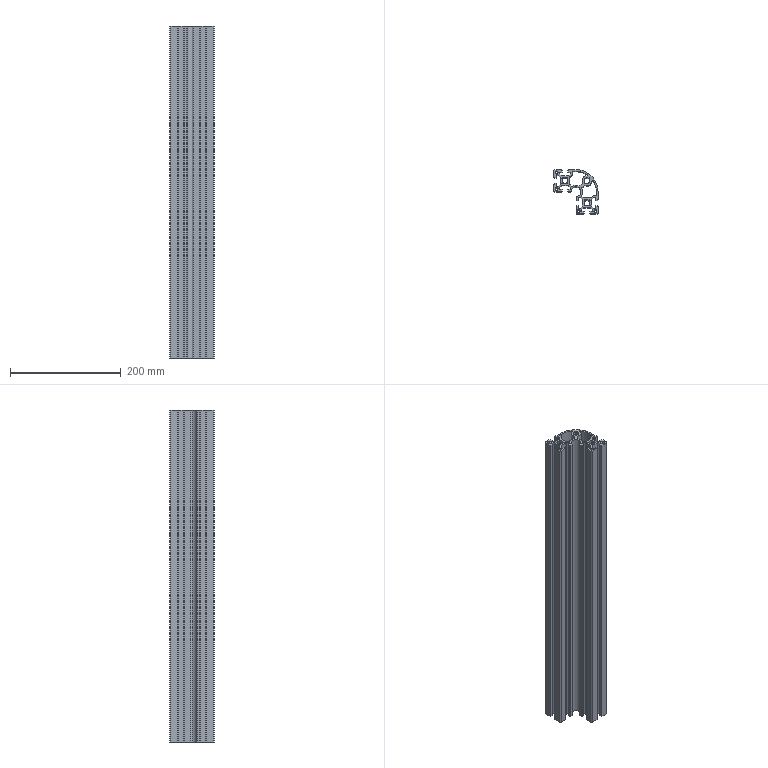Part | SolidWorks | features Extrusion 1 | 1 solid | 229 faces | box 80 x 80 x 600 mm | volume 1006193 mm3 | plane 124 | cylinder 105 | commonest cylinder face diameters 2 x71 10.2 x13 5 x8 4 x4 18 x4 24 x2